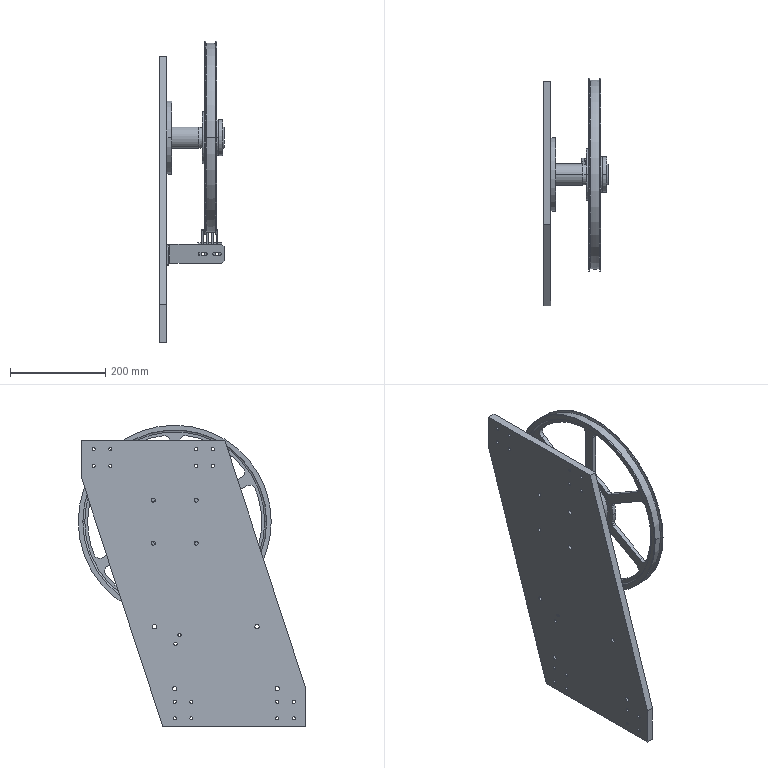Part | SolidWorks | 15 solids | 917 faces | box 135 x 477.5 x 632.5 mm | volume 3947731 mm3 | cylinder 449 | plane 188 | sphere 132 | torus 100 | cone 48 | commonest cylinder face diameters 11 x48 6.6 x44 0.4 x40 5 x36 15 x26 1.57 x24